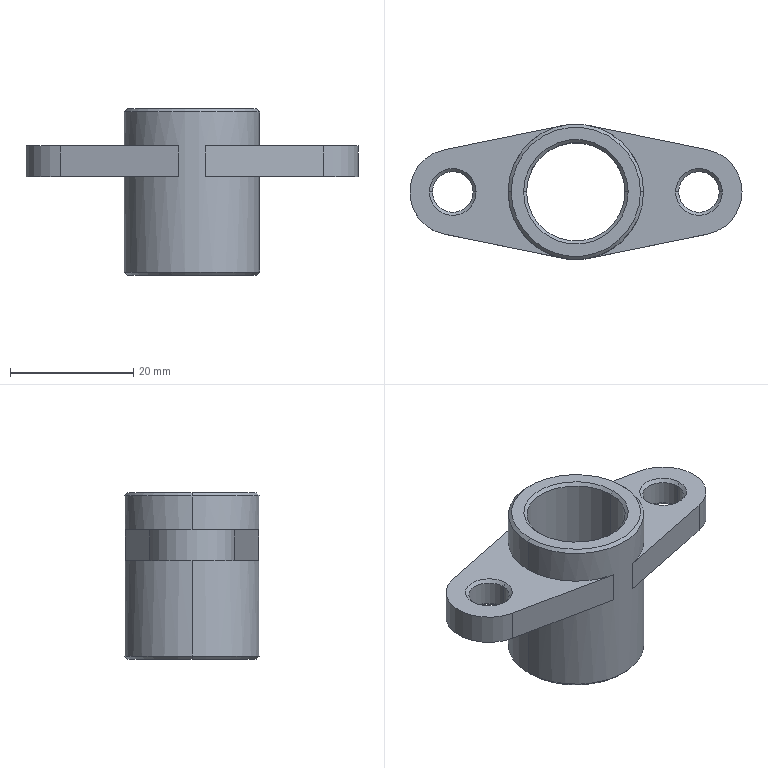Part | SolidWorks | features ICE 3, 3DProfileFeature 1, Chamfer 1, Extrusion 1, HoleWzd 1 | 1 solid | 37 faces | box 54 x 22 x 27 mm | volume 6993 mm3 | cone 16 | cylinder 11 | plane 10 | commonest cylinder face diameters 6.6 x4 14 x3 16 x2 22 x2
STEP:
#1=CARTESIAN_POINT('',(-10.5,0.,0.));
#2=VERTEX_POINT('',#1);
#3=CARTESIAN_POINT('',(10.5,0.,0.));
#4=VERTEX_POINT('',#3);
#5=CARTESIAN_POINT('',(0.,0.,0.));
#6=DIRECTION('',(0.,0.,-1.));
#7=DIRECTION('',(1.,0.,0.));
#8=AXIS2_PLACEMENT_3D('',#5,#6,#7);
#9=CIRCLE('',#8,10.5);
#10=EDGE_CURVE('',#2,#4,#9,.T.);
#11=ORIENTED_EDGE('',*,*,#10,.F.);
#12=CARTESIAN_POINT('',(-11.,0.,0.5));
#13=VERTEX_POINT('',#12);
#14=CARTESIAN_POINT('',(-11.,0.,0.5));
#15=DIRECTION('',(-0.7071,0.,0.7071));
#16=VECTOR('',#15,1000.);
#17=LINE('',#14,#16);
#18=EDGE_CURVE('',#2,#13,#17,.T.);
#19=ORIENTED_EDGE('',*,*,#18,.T.);
#20=CARTESIAN_POINT('',(11.,0.,0.5));
#21=VERTEX_POINT('',#20);
#22=CARTESIAN_POINT('',(0.,0.,0.5));
#23=DIRECTION('',(0.,0.,1.));
#24=DIRECTION('',(1.,0.,0.));
#25=AXIS2_PLACEMENT_3D('',#22,#23,#24);
#26=CIRCLE('',#25,11.);
#27=EDGE_CURVE('',#21,#13,#26,.T.);
#28=ORIENTED_EDGE('',*,*,#27,.F.);
#29=CARTESIAN_POINT('',(11.,0.,0.5));
#30=DIRECTION('',(0.7071,0.,0.7071));
#31=VECTOR('',#30,1000.);
#32=LINE('',#29,#31);
#33=EDGE_CURVE('',#4,#21,#32,.T.);
#34=ORIENTED_EDGE('',*,*,#33,.F.);
#35=EDGE_LOOP('',(#11,#19,#28,#34));
#36=FACE_OUTER_BOUND('',#35,.T.);
#37=CARTESIAN_POINT('',(0.,0.,0.5));
#38=DIRECTION('',(0.,0.,1.));
#39=DIRECTION('',(1.,0.,0.));
#40=AXIS2_PLACEMENT_3D('',#37,#38,#39);
#41=CONICAL_SURFACE('',#40,11.,0.7854);
#42=ADVANCED_FACE('',(#36),#41,.T.);
#43=CARTESIAN_POINT('',(8.,0.,0.5));
#44=VERTEX_POINT('',#43);
#45=CARTESIAN_POINT('',(-8.,0.,0.5));
#46=VERTEX_POINT('',#45);
#47=CARTESIAN_POINT('',(0.,0.,0.5));
#48=DIRECTION('',(0.,0.,-1.));
#49=DIRECTION('',(1.,0.,0.));
#50=AXIS2_PLACEMENT_3D('',#47,#48,#49);
#51=CIRCLE('',#50,8.);
#52=EDGE_CURVE('',#44,#46,#51,.T.);
#53=ORIENTED_EDGE('',*,*,#52,.F.);
#54=CARTESIAN_POINT('',(8.5,0.,0.));
#55=VERTEX_POINT('',#54);
#56=CARTESIAN_POINT('',(8.5,0.,0.));
#57=DIRECTION('',(0.7071,0.,-0.7071));
#58=VECTOR('',#57,1000.);
#59=LINE('',#56,#58);
#60=EDGE_CURVE('',#44,#55,#59,.T.);
#61=ORIENTED_EDGE('',*,*,#60,.T.);
#62=CARTESIAN_POINT('',(-8.5,0.,0.));
#63=VERTEX_POINT('',#62);
#64=CARTESIAN_POINT('',(0.,0.,0.));
#65=DIRECTION('',(0.,0.,1.));
#66=DIRECTION('',(1.,0.,0.));
#67=AXIS2_PLACEMENT_3D('',#64,#65,#66);
#68=CIRCLE('',#67,8.5);
#69=EDGE_CURVE('',#63,#55,#68,.T.);
#70=ORIENTED_EDGE('',*,*,#69,.F.);
#71=CARTESIAN_POINT('',(-8.5,0.,0.));
#72=DIRECTION('',(-0.7071,0.,-0.7071));
#73=VECTOR('',#72,1000.);
#74=LINE('',#71,#73);
#75=EDGE_CURVE('',#46,#63,#74,.T.);
#76=ORIENTED_EDGE('',*,*,#75,.F.);
#77=EDGE_LOOP('',(#53,#61,#70,#76));
#78=FACE_OUTER_BOUND('',#77,.T.);
#79=CARTESIAN_POINT('',(0.,0.,0.));
#80=DIRECTION('',(0.,0.,-1.));
#81=DIRECTION('',(-1.,0.,0.));
#82=AXIS2_PLACEMENT_3D('',#79,#80,#81);
#83=CONICAL_SURFACE('',#82,8.5,0.7854);
#84=ADVANCED_FACE('',(#78),#83,.F.);
#85=CARTESIAN_POINT('',(-16.7,0.,16.5));
#86=VERTEX_POINT('',#85);
#87=CARTESIAN_POINT('',(-23.3,0.,16.5));
#88=VERTEX_POINT('',#87);
#89=CARTESIAN_POINT('',(-20.,0.,16.5));
#90=DIRECTION('',(0.,0.,-1.));
#91=DIRECTION('',(1.,0.,0.));
#92=AXIS2_PLACEMENT_3D('',#89,#90,#91);
#93=CIRCLE('',#92,3.3);
#94=EDGE_CURVE('',#86,#88,#93,.T.);
#95=ORIENTED_EDGE('',*,*,#94,.F.);
#96=CARTESIAN_POINT('',(-16.2,0.,16.));
#97=VERTEX_POINT('',#96);
#98=CARTESIAN_POINT('',(-16.2,0.,16.));
#99=DIRECTION('',(0.7071,0.,-0.7071));
#100=VECTOR('',#99,1000.);
#101=LINE('',#98,#100);
#102=EDGE_CURVE('',#86,#97,#101,.T.);
#103=ORIENTED_EDGE('',*,*,#102,.T.);
#104=CARTESIAN_POINT('',(-23.8,0.,16.));
#105=VERTEX_POINT('',#104);
#106=CARTESIAN_POINT('',(-20.,0.,16.));
#107=DIRECTION('',(0.,0.,1.));
#108=DIRECTION('',(1.,0.,0.));
#109=AXIS2_PLACEMENT_3D('',#106,#107,#108);
#110=CIRCLE('',#109,3.8);
#111=EDGE_CURVE('',#105,#97,#110,.T.);
#112=ORIENTED_EDGE('',*,*,#111,.F.);
#113=CARTESIAN_POINT('',(-23.8,0.,16.));
#114=DIRECTION('',(-0.7071,0.,-0.7071));
#115=VECTOR('',#114,1000.);
#116=LINE('',#113,#115);
#117=EDGE_CURVE('',#88,#105,#116,.T.);
#118=ORIENTED_EDGE('',*,*,#117,.F.);
#119=EDGE_LOOP('',(#95,#103,#112,#118));
#120=FACE_OUTER_BOUND('',#119,.T.);
#121=CARTESIAN_POINT('',(-20.,0.,16.));
#122=DIRECTION('',(0.,0.,-1.));
#123=DIRECTION('',(-1.,0.,0.));
#124=AXIS2_PLACEMENT_3D('',#121,#122,#123);
#125=CONICAL_SURFACE('',#124,3.8,0.7854);
#126=ADVANCED_FACE('',(#120),#125,.F.);
#127=CARTESIAN_POINT('',(-23.3,0.,20.5));
#128=VERTEX_POINT('',#127);
#129=CARTESIAN_POINT('',(-16.7,0.,20.5));
#130=VERTEX_POINT('',#129);
#131=CARTESIAN_POINT('',(-20.,0.,20.5));
#132=DIRECTION('',(0.,0.,1.));
#133=DIRECTION('',(-1.,0.,0.));
#134=AXIS2_PLACEMENT_3D('',#131,#132,#133);
#135=CIRCLE('',#134,3.3);
#136=EDGE_CURVE('',#128,#130,#135,.T.);
#137=ORIENTED_EDGE('',*,*,#136,.F.);
#138=CARTESIAN_POINT('',(-23.8,0.,21.));
#139=VERTEX_POINT('',#138);
#140=CARTESIAN_POINT('',(-23.3,0.,20.5));
#141=DIRECTION('',(-0.7071,0.,0.7071));
#142=VECTOR('',#141,1000.);
#143=LINE('',#140,#142);
#144=EDGE_CURVE('',#128,#139,#143,.T.);
#145=ORIENTED_EDGE('',*,*,#144,.T.);
#146=CARTESIAN_POINT('',(-16.2,0.,21.));
#147=VERTEX_POINT('',#146);
#148=CARTESIAN_POINT('',(-20.,0.,21.));
#149=DIRECTION('',(0.,0.,-1.));
#150=DIRECTION('',(-1.,0.,0.));
#151=AXIS2_PLACEMENT_3D('',#148,#149,#150);
#152=CIRCLE('',#151,3.8);
#153=EDGE_CURVE('',#147,#139,#152,.T.);
#154=ORIENTED_EDGE('',*,*,#153,.F.);
#155=CARTESIAN_POINT('',(-16.7,0.,20.5));
#156=DIRECTION('',(0.7071,0.,0.7071));
#157=VECTOR('',#156,1000.);
#158=LINE('',#155,#157);
#159=EDGE_CURVE('',#130,#147,#158,.T.);
#160=ORIENTED_EDGE('',*,*,#159,.F.);
#161=EDGE_LOOP('',(#137,#145,#154,#160));
#162=FACE_OUTER_BOUND('',#161,.T.);
#163=CARTESIAN_POINT('',(-20.,0.,20.5));
#164=DIRECTION('',(0.,0.,1.));
#165=DIRECTION('',(1.,0.,0.));
#166=AXIS2_PLACEMENT_3D('',#163,#164,#165);
#167=CONICAL_SURFACE('',#166,3.3,0.7854);
#168=ADVANCED_FACE('',(#162),#167,.F.);
#169=CARTESIAN_POINT('',(23.3,0.,16.5));
#170=VERTEX_POINT('',#169);
#171=CARTESIAN_POINT('',(16.7,0.,16.5));
#172=VERTEX_POINT('',#171);
#173=CARTESIAN_POINT('',(20.,0.,16.5));
#174=DIRECTION('',(0.,0.,-1.));
#175=DIRECTION('',(1.,0.,0.));
#176=AXIS2_PLACEMENT_3D('',#173,#174,#175);
#177=CIRCLE('',#176,3.3);
#178=EDGE_CURVE('',#170,#172,#177,.T.);
#179=ORIENTED_EDGE('',*,*,#178,.F.);
#180=CARTESIAN_POINT('',(23.8,0.,16.));
#181=VERTEX_POINT('',#180);
#182=CARTESIAN_POINT('',(23.8,0.,16.));
#183=DIRECTION('',(0.7071,0.,-0.7071));
#184=VECTOR('',#183,1000.);
#185=LINE('',#182,#184);
#186=EDGE_CURVE('',#170,#181,#185,.T.);
#187=ORIENTED_EDGE('',*,*,#186,.T.);
#188=CARTESIAN_POINT('',(16.2,0.,16.));
#189=VERTEX_POINT('',#188);
#190=CARTESIAN_POINT('',(20.,0.,16.));
#191=DIRECTION('',(0.,0.,1.));
#192=DIRECTION('',(1.,0.,0.));
#193=AXIS2_PLACEMENT_3D('',#190,#191,#192);
#194=CIRCLE('',#193,3.8);
#195=EDGE_CURVE('',#189,#181,#194,.T.);
#196=ORIENTED_EDGE('',*,*,#195,.F.);
#197=CARTESIAN_POINT('',(16.2,0.,16.));
#198=DIRECTION('',(-0.7071,0.,-0.7071));
#199=VECTOR('',#198,1000.);
#200=LINE('',#197,#199);
#201=EDGE_CURVE('',#172,#189,#200,.T.);
#202=ORIENTED_EDGE('',*,*,#201,.F.);
#203=EDGE_LOOP('',(#179,#187,#196,#202));
#204=FACE_OUTER_BOUND('',#203,.T.);
#205=CARTESIAN_POINT('',(20.,0.,16.));
#206=DIRECTION('',(0.,0.,-1.));
#207=DIRECTION('',(-1.,0.,0.));
#208=AXIS2_PLACEMENT_3D('',#205,#206,#207);
#209=CONICAL_SURFACE('',#208,3.8,0.7854);
#210=ADVANCED_FACE('',(#204),#209,.F.);
#211=CARTESIAN_POINT('',(16.7,0.,20.5));
#212=VERTEX_POINT('',#211);
#213=CARTESIAN_POINT('',(23.3,0.,20.5));
#214=VERTEX_POINT('',#213);
#215=CARTESIAN_POINT('',(20.,0.,20.5));
#216=DIRECTION('',(0.,0.,1.));
#217=DIRECTION('',(-1.,0.,0.));
#218=AXIS2_PLACEMENT_3D('',#215,#216,#217);
#219=CIRCLE('',#218,3.3);
#220=EDGE_CURVE('',#212,#214,#219,.T.);
#221=ORIENTED_EDGE('',*,*,#220,.F.);
#222=CARTESIAN_POINT('',(16.2,0.,21.));
#223=VERTEX_POINT('',#222);
#224=CARTESIAN_POINT('',(16.7,0.,20.5));
#225=DIRECTION('',(-0.7071,0.,0.7071));
#226=VECTOR('',#225,1000.);
#227=LINE('',#224,#226);
#228=EDGE_CURVE('',#212,#223,#227,.T.);
#229=ORIENTED_EDGE('',*,*,#228,.T.);
#230=CARTESIAN_POINT('',(23.8,0.,21.));
#231=VERTEX_POINT('',#230);
#232=CARTESIAN_POINT('',(20.,0.,21.));
#233=DIRECTION('',(0.,0.,-1.));
#234=DIRECTION('',(-1.,0.,0.));
#235=AXIS2_PLACEMENT_3D('',#232,#233,#234);
#236=CIRCLE('',#235,3.8);
#237=EDGE_CURVE('',#231,#223,#236,.T.);
#238=ORIENTED_EDGE('',*,*,#237,.F.);
#239=CARTESIAN_POINT('',(23.3,0.,20.5));
#240=DIRECTION('',(0.7071,0.,0.7071));
#241=VECTOR('',#240,1000.);
#242=LINE('',#239,#241);
#243=EDGE_CURVE('',#214,#231,#242,.T.);
#244=ORIENTED_EDGE('',*,*,#243,.F.);
#245=EDGE_LOOP('',(#221,#229,#238,#244));
#246=FACE_OUTER_BOUND('',#245,.T.);
#247=CARTESIAN_POINT('',(20.,0.,20.5));
#248=DIRECTION('',(0.,0.,1.));
#249=DIRECTION('',(1.,0.,0.));
#250=AXIS2_PLACEMENT_3D('',#247,#248,#249);
#251=CONICAL_SURFACE('',#250,3.3,0.7854);
#252=ADVANCED_FACE('',(#246),#251,.F.);
#253=CARTESIAN_POINT('',(-8.,0.,26.5));
#254=VERTEX_POINT('',#253);
#255=CARTESIAN_POINT('',(8.,0.,26.5));
#256=VERTEX_POINT('',#255);
#257=CARTESIAN_POINT('',(0.,0.,26.5));
#258=DIRECTION('',(0.,0.,1.));
#259=DIRECTION('',(1.,0.,0.));
#260=AXIS2_PLACEMENT_3D('',#257,#258,#259);
#261=CIRCLE('',#260,8.);
#262=EDGE_CURVE('',#254,#256,#261,.T.);
#263=ORIENTED_EDGE('',*,*,#262,.F.);
#264=CARTESIAN_POINT('',(-8.5,0.,27.));
#265=VERTEX_POINT('',#264);
#266=CARTESIAN_POINT('',(-8.,0.,26.5));
#267=DIRECTION('',(-0.7071,0.,0.7071));
#268=VECTOR('',#267,1000.);
#269=LINE('',#266,#268);
#270=EDGE_CURVE('',#254,#265,#269,.T.);
#271=ORIENTED_EDGE('',*,*,#270,.T.);
#272=CARTESIAN_POINT('',(8.5,0.,27.));
#273=VERTEX_POINT('',#272);
#274=CARTESIAN_POINT('',(0.,0.,27.));
#275=DIRECTION('',(0.,0.,-1.));
#276=DIRECTION('',(1.,0.,0.));
#277=AXIS2_PLACEMENT_3D('',#274,#275,#276);
#278=CIRCLE('',#277,8.5);
#279=EDGE_CURVE('',#273,#265,#278,.T.);
#280=ORIENTED_EDGE('',*,*,#279,.F.);
#281=CARTESIAN_POINT('',(8.,0.,26.5));
#282=DIRECTION('',(0.7071,0.,0.7071));
#283=VECTOR('',#282,1000.);
#284=LINE('',#281,#283);
#285=EDGE_CURVE('',#256,#273,#284,.T.);
#286=ORIENTED_EDGE('',*,*,#285,.F.);
#287=EDGE_LOOP('',(#263,#271,#280,#286));
#288=FACE_OUTER_BOUND('',#287,.T.);
#289=CARTESIAN_POINT('',(0.,0.,26.5));
#290=DIRECTION('',(0.,0.,1.));
#291=DIRECTION('',(1.,0.,0.));
#292=AXIS2_PLACEMENT_3D('',#289,#290,#291);
#293=CONICAL_SURFACE('',#292,8.,0.7854);
#294=ADVANCED_FACE('',(#288),#293,.F.);
#295=CARTESIAN_POINT('',(10.5,0.,27.));
#296=VERTEX_POINT('',#295);
#297=CARTESIAN_POINT('',(-10.5,0.,27.));
#298=VERTEX_POINT('',#297);
#299=CARTESIAN_POINT('',(0.,0.,27.));
#300=DIRECTION('',(0.,0.,1.));
#301=DIRECTION('',(1.,0.,0.));
#302=AXIS2_PLACEMENT_3D('',#299,#300,#301);
#303=CIRCLE('',#302,10.5);
#304=EDGE_CURVE('',#296,#298,#303,.T.);
#305=ORIENTED_EDGE('',*,*,#304,.F.);
#306=CARTESIAN_POINT('',(11.,0.,26.5));
#307=VERTEX_POINT('',#306);
#308=CARTESIAN_POINT('',(10.5,0.,27.));
#309=DIRECTION('',(0.7071,0.,-0.7071));
#310=VECTOR('',#309,1000.);
#311=LINE('',#308,#310);
#312=EDGE_CURVE('',#296,#307,#311,.T.);
#313=ORIENTED_EDGE('',*,*,#312,.T.);
#314=CARTESIAN_POINT('',(-11.,0.,26.5));
#315=VERTEX_POINT('',#314);
#316=CARTESIAN_POINT('',(0.,0.,26.5));
#317=DIRECTION('',(0.,0.,-1.));
#318=DIRECTION('',(1.,0.,0.));
#319=AXIS2_PLACEMENT_3D('',#316,#317,#318);
#320=CIRCLE('',#319,11.);
#321=EDGE_CURVE('',#315,#307,#320,.T.);
#322=ORIENTED_EDGE('',*,*,#321,.F.);
#323=CARTESIAN_POINT('',(-10.5,0.,27.));
#324=DIRECTION('',(-0.7071,0.,-0.7071));
#325=VECTOR('',#324,1000.);
#326=LINE('',#323,#325);
#327=EDGE_CURVE('',#298,#315,#326,.T.);
#328=ORIENTED_EDGE('',*,*,#327,.F.);
#329=EDGE_LOOP('',(#305,#313,#322,#328));
#330=FACE_OUTER_BOUND('',#329,.T.);
#331=CARTESIAN_POINT('',(0.,0.,27.));
#332=DIRECTION('',(0.,0.,-1.));
#333=DIRECTION('',(-1.,0.,0.));
#334=AXIS2_PLACEMENT_3D('',#331,#332,#333);
#335=CONICAL_SURFACE('',#334,10.5,0.7854);
#336=ADVANCED_FACE('',(#330),#335,.T.);
#337=ORIENTED_EDGE('',*,*,#94,.T.);
#338=CARTESIAN_POINT('',(-23.3,0.,30.));
#339=DIRECTION('',(0.,0.,1.));
#340=VECTOR('',#339,1000.);
#341=LINE('',#338,#340);
#342=EDGE_CURVE('',#88,#128,#341,.T.);
#343=ORIENTED_EDGE('',*,*,#342,.T.);
#344=ORIENTED_EDGE('',*,*,#136,.T.);
#345=CARTESIAN_POINT('',(-16.7,0.,30.));
#346=DIRECTION('',(0.,0.,1.));
#347=VECTOR('',#346,1000.);
#348=LINE('',#345,#347);
#349=EDGE_CURVE('',#86,#130,#348,.T.);
#350=ORIENTED_EDGE('',*,*,#349,.F.);
#351=EDGE_LOOP('',(#337,#343,#344,#350));
#352=FACE_OUTER_BOUND('',#351,.T.);
#353=CARTESIAN_POINT('',(-20.,0.,30.));
#354=DIRECTION('',(0.,0.,1.));
#355=DIRECTION('',(1.,0.,0.));
#356=AXIS2_PLACEMENT_3D('',#353,#354,#355);
#357=CYLINDRICAL_SURFACE('',#356,3.3);
#358=ADVANCED_FACE('',(#352),#357,.F.);
#359=ORIENTED_EDGE('',*,*,#178,.T.);
#360=CARTESIAN_POINT('',(16.7,0.,30.));
#361=DIRECTION('',(0.,0.,1.));
#362=VECTOR('',#361,1000.);
#363=LINE('',#360,#362);
#364=EDGE_CURVE('',#172,#212,#363,.T.);
#365=ORIENTED_EDGE('',*,*,#364,.T.);
#366=ORIENTED_EDGE('',*,*,#220,.T.);
#367=CARTESIAN_POINT('',(23.3,0.,30.));
#368=DIRECTION('',(0.,0.,1.));
#369=VECTOR('',#368,1000.);
#370=LINE('',#367,#369);
#371=EDGE_CURVE('',#170,#214,#370,.T.);
#372=ORIENTED_EDGE('',*,*,#371,.F.);
#373=EDGE_LOOP('',(#359,#365,#366,#372));
#374=FACE_OUTER_BOUND('',#373,.T.);
#375=CARTESIAN_POINT('',(20.,0.,30.));
#376=DIRECTION('',(0.,0.,1.));
#377=DIRECTION('',(1.,0.,0.));
#378=AXIS2_PLACEMENT_3D('',#375,#376,#377);
#379=CYLINDRICAL_SURFACE('',#378,3.3);
#380=ADVANCED_FACE('',(#374),#379,.F.);
#381=CARTESIAN_POINT('',(21.4,-6.859,16.));
#382=VERTEX_POINT('',#381);
#383=CARTESIAN_POINT('',(27.,0.,16.));
#384=VERTEX_POINT('',#383);
#385=CARTESIAN_POINT('',(20.,0.,16.));
#386=DIRECTION('',(0.,0.,1.));
#387=DIRECTION('',(1.,0.,0.));
#388=AXIS2_PLACEMENT_3D('',#385,#386,#387);
#389=CIRCLE('',#388,7.);
#390=EDGE_CURVE('',#382,#384,#389,.T.);
#391=ORIENTED_EDGE('',*,*,#390,.T.);
#392=CARTESIAN_POINT('',(27.,0.,21.));
#393=VERTEX_POINT('',#392);
#394=CARTESIAN_POINT('',(27.,0.,16.));
#395=DIRECTION('',(0.,0.,1.));
#396=VECTOR('',#395,1000.);
#397=LINE('',#394,#396);
#398=EDGE_CURVE('',#384,#393,#397,.T.);
#399=ORIENTED_EDGE('',*,*,#398,.T.);
#400=CARTESIAN_POINT('',(21.4,-6.859,21.));
#401=VERTEX_POINT('',#400);
#402=CARTESIAN_POINT('',(20.,0.,21.));
#403=DIRECTION('',(0.,0.,1.));
#404=DIRECTION('',(-1.,0.,0.));
#405=AXIS2_PLACEMENT_3D('',#402,#403,#404);
#406=CIRCLE('',#405,7.);
#407=EDGE_CURVE('',#401,#393,#406,.T.);
#408=ORIENTED_EDGE('',*,*,#407,.F.);
#409=CARTESIAN_POINT('',(21.4,-6.859,16.));
#410=DIRECTION('',(0.,0.,1.));
#411=VECTOR('',#410,1000.);
#412=LINE('',#409,#411);
#413=EDGE_CURVE('',#382,#401,#412,.T.);
#414=ORIENTED_EDGE('',*,*,#413,.F.);
#415=EDGE_LOOP('',(#391,#399,#408,#414));
#416=FACE_OUTER_BOUND('',#415,.T.);
#417=CARTESIAN_POINT('',(20.,0.,16.));
#418=DIRECTION('',(0.,0.,1.));
#419=DIRECTION('',(1.,0.,0.));
#420=AXIS2_PLACEMENT_3D('',#417,#418,#419);
#421=CYLINDRICAL_SURFACE('',#420,7.);
#422=ADVANCED_FACE('',(#416),#421,.T.);
#423=ORIENTED_EDGE('',*,*,#262,.T.);
#424=CARTESIAN_POINT('',(8.,0.,30.));
#425=DIRECTION('',(0.,0.,-1.));
#426=VECTOR('',#425,1000.);
#427=LINE('',#424,#426);
#428=EDGE_CURVE('',#256,#44,#427,.T.);
#429=ORIENTED_EDGE('',*,*,#428,.T.);
#430=ORIENTED_EDGE('',*,*,#52,.T.);
#431=CARTESIAN_POINT('',(-8.,0.,30.));
#432=DIRECTION('',(0.,0.,-1.));
#433=VECTOR('',#432,1000.);
#434=LINE('',#431,#433);
#435=EDGE_CURVE('',#254,#46,#434,.T.);
#436=ORIENTED_EDGE('',*,*,#435,.F.);
#437=EDGE_LOOP('',(#423,#429,#430,#436));
#438=FACE_OUTER_BOUND('',#437,.T.);
#439=CARTESIAN_POINT('',(0.,0.,30.));
#440=DIRECTION('',(0.,0.,-1.));
#441=DIRECTION('',(-1.,0.,0.));
#442=AXIS2_PLACEMENT_3D('',#439,#440,#441);
#443=CYLINDRICAL_SURFACE('',#442,8.);
#444=ADVANCED_FACE('',(#438),#443,.F.);
#445=ORIENTED_EDGE('',*,*,#321,.T.);
#446=CARTESIAN_POINT('',(11.,0.,21.));
#447=VERTEX_POINT('',#446);
#448=CARTESIAN_POINT('',(11.,0.,30.));
#449=DIRECTION('',(0.,0.,-1.));
#450=VECTOR('',#449,1000.);
#451=LINE('',#448,#450);
#452=EDGE_CURVE('',#307,#447,#451,.T.);
#453=ORIENTED_EDGE('',*,*,#452,.T.);
#454=CARTESIAN_POINT('',(2.2,10.778,21.));
#455=VERTEX_POINT('',#454);
#456=CARTESIAN_POINT('',(0.,0.,21.));
#457=DIRECTION('',(0.,0.,1.));
#458=DIRECTION('',(-1.,0.,0.));
#459=AXIS2_PLACEMENT_3D('',#456,#457,#458);
#460=CIRCLE('',#459,11.);
#461=EDGE_CURVE('',#447,#455,#460,.T.);
#462=ORIENTED_EDGE('',*,*,#461,.T.);
#463=CARTESIAN_POINT('',(2.2,10.778,16.));
#464=VERTEX_POINT('',#463);
#465=CARTESIAN_POINT('',(2.2,10.778,16.));
#466=DIRECTION('',(0.,0.,1.));
#467=VECTOR('',#466,1000.);
#468=LINE('',#465,#467);
#469=EDGE_CURVE('',#464,#455,#468,.T.);
#470=ORIENTED_EDGE('',*,*,#469,.F.);
#471=CARTESIAN_POINT('',(11.,0.,16.));
#472=VERTEX_POINT('',#471);
#473=CARTESIAN_POINT('',(0.,0.,16.));
#474=DIRECTION('',(0.,0.,1.));
#475=DIRECTION('',(1.,0.,0.));
#476=AXIS2_PLACEMENT_3D('',#473,#474,#475);
#477=CIRCLE('',#476,11.);
#478=EDGE_CURVE('',#472,#464,#477,.T.);
#479=ORIENTED_EDGE('',*,*,#478,.F.);
#480=CARTESIAN_POINT('',(11.,0.,30.));
#481=DIRECTION('',(0.,0.,-1.));
#482=VECTOR('',#481,1000.);
#483=LINE('',#480,#482);
#484=EDGE_CURVE('',#472,#21,#483,.T.);
#485=ORIENTED_EDGE('',*,*,#484,.T.);
#486=ORIENTED_EDGE('',*,*,#27,.T.);
#487=CARTESIAN_POINT('',(-11.,0.,16.));
#488=VERTEX_POINT('',#487);
#489=CARTESIAN_POINT('',(-11.,0.,30.));
#490=DIRECTION('',(0.,0.,-1.));
#491=VECTOR('',#490,1000.);
#492=LINE('',#489,#491);
#493=EDGE_CURVE('',#488,#13,#492,.T.);
#494=ORIENTED_EDGE('',*,*,#493,.F.);
#495=CARTESIAN_POINT('',(-2.2,10.778,16.));
#496=VERTEX_POINT('',#495);
#497=CARTESIAN_POINT('',(0.,0.,16.));
#498=DIRECTION('',(0.,0.,1.));
#499=DIRECTION('',(1.,0.,0.));
#500=AXIS2_PLACEMENT_3D('',#497,#498,#499);
#501=CIRCLE('',#500,11.);
#502=EDGE_CURVE('',#496,#488,#501,.T.);
#503=ORIENTED_EDGE('',*,*,#502,.F.);
#504=CARTESIAN_POINT('',(-2.2,10.778,21.));
#505=VERTEX_POINT('',#504);
#506=CARTESIAN_POINT('',(-2.2,10.778,16.));
#507=DIRECTION('',(0.,0.,1.));
#508=VECTOR('',#507,1000.);
#509=LINE('',#506,#508);
#510=EDGE_CURVE('',#496,#505,#509,.T.);
#511=ORIENTED_EDGE('',*,*,#510,.T.);
#512=CARTESIAN_POINT('',(-11.,0.,21.));
#513=VERTEX_POINT('',#512);
#514=CARTESIAN_POINT('',(0.,0.,21.));
#515=DIRECTION('',(0.,0.,1.));
#516=DIRECTION('',(-1.,0.,0.));
#517=AXIS2_PLACEMENT_3D('',#514,#515,#516);
#518=CIRCLE('',#517,11.);
#519=EDGE_CURVE('',#505,#513,#518,.T.);
#520=ORIENTED_EDGE('',*,*,#519,.T.);
#521=CARTESIAN_POINT('',(-11.,0.,30.));
#522=DIRECTION('',(0.,0.,-1.));
#523=VECTOR('',#522,1000.);
#524=LINE('',#521,#523);
#525=EDGE_CURVE('',#315,#513,#524,.T.);
#526=ORIENTED_EDGE('',*,*,#525,.F.);
#527=EDGE_LOOP('',(#445,#453,#462,#470,#479,#485,#486,#494,#503,#511,#520,#526));
#528=FACE_OUTER_BOUND('',#527,.T.);
#529=CARTESIAN_POINT('',(0.,0.,30.));
#530=DIRECTION('',(0.,0.,-1.));
#531=DIRECTION('',(-1.,0.,0.));
#532=AXIS2_PLACEMENT_3D('',#529,#530,#531);
#533=CYLINDRICAL_SURFACE('',#532,11.);
#534=ADVANCED_FACE('',(#528),#533,.T.);
#535=ORIENTED_EDGE('',*,*,#452,.F.);
#536=CARTESIAN_POINT('',(0.,0.,26.5));
#537=DIRECTION('',(0.,0.,-1.));
#538=DIRECTION('',(1.,0.,0.));
#539=AXIS2_PLACEMENT_3D('',#536,#537,#538);
#540=CIRCLE('',#539,11.);
#541=EDGE_CURVE('',#307,#315,#540,.T.);
#542=ORIENTED_EDGE('',*,*,#541,.T.);
#543=ORIENTED_EDGE('',*,*,#525,.T.);
#544=CARTESIAN_POINT('',(-2.2,-10.778,21.));
#545=VERTEX_POINT('',#544);
#546=CARTESIAN_POINT('',(0.,0.,21.));
#547=DIRECTION('',(0.,0.,1.));
#548=DIRECTION('',(-1.,0.,0.));
#549=AXIS2_PLACEMENT_3D('',#546,#547,#548);
#550=CIRCLE('',#549,11.);
#551=EDGE_CURVE('',#513,#545,#550,.T.);
#552=ORIENTED_EDGE('',*,*,#551,.T.);
#553=CARTESIAN_POINT('',(-2.2,-10.778,16.));
#554=VERTEX_POINT('',#553);
#555=CARTESIAN_POINT('',(-2.2,-10.778,16.));
#556=DIRECTION('',(0.,0.,1.));
#557=VECTOR('',#556,1000.);
#558=LINE('',#555,#557);
#559=EDGE_CURVE('',#554,#545,#558,.T.);
#560=ORIENTED_EDGE('',*,*,#559,.F.);
#561=CARTESIAN_POINT('',(0.,0.,16.));
#562=DIRECTION('',(0.,0.,1.));
#563=DIRECTION('',(1.,0.,0.));
#564=AXIS2_PLACEMENT_3D('',#561,#562,#563);
#565=CIRCLE('',#564,11.);
#566=EDGE_CURVE('',#488,#554,#565,.T.);
#567=ORIENTED_EDGE('',*,*,#566,.F.);
#568=ORIENTED_EDGE('',*,*,#493,.T.);
#569=CARTESIAN_POINT('',(0.,0.,0.5));
#570=DIRECTION('',(0.,0.,1.));
#571=DIRECTION('',(1.,0.,0.));
#572=AXIS2_PLACEMENT_3D('',#569,#570,#571);
#573=CIRCLE('',#572,11.);
#574=EDGE_CURVE('',#13,#21,#573,.T.);
#575=ORIENTED_EDGE('',*,*,#574,.T.);
#576=ORIENTED_EDGE('',*,*,#484,.F.);
#577=CARTESIAN_POINT('',(2.2,-10.778,16.));
#578=VERTEX_POINT('',#577);
#579=CARTESIAN_POINT('',(0.,0.,16.));
#580=DIRECTION('',(0.,0.,1.));
#581=DIRECTION('',(1.,0.,0.));
#582=AXIS2_PLACEMENT_3D('',#579,#580,#581);
#583=CIRCLE('',#582,11.);
#584=EDGE_CURVE('',#578,#472,#583,.T.);
#585=ORIENTED_EDGE('',*,*,#584,.F.);
#586=CARTESIAN_POINT('',(2.2,-10.778,21.));
#587=VERTEX_POINT('',#586);
#588=CARTESIAN_POINT('',(2.2,-10.778,16.));
#589=DIRECTION('',(0.,0.,1.));
#590=VECTOR('',#589,1000.);
#591=LINE('',#588,#590);
#592=EDGE_CURVE('',#578,#587,#591,.T.);
#593=ORIENTED_EDGE('',*,*,#592,.T.);
#594=CARTESIAN_POINT('',(0.,0.,21.));
#595=DIRECTION('',(0.,0.,1.));
#596=DIRECTION('',(-1.,0.,0.));
#597=AXIS2_PLACEMENT_3D('',#594,#595,#596);
#598=CIRCLE('',#597,11.);
#599=EDGE_CURVE('',#587,#447,#598,.T.);
#600=ORIENTED_EDGE('',*,*,#599,.T.);
#601=EDGE_LOOP('',(#535,#542,#543,#552,#560,#567,#568,#575,#576,#585,#593,#600));
#602=FACE_OUTER_BOUND('',#601,.T.);
#603=CARTESIAN_POINT('',(0.,0.,30.));
#604=DIRECTION('',(0.,0.,-1.));
#605=DIRECTION('',(-1.,0.,0.));
#606=AXIS2_PLACEMENT_3D('',#603,#604,#605);
#607=CYLINDRICAL_SURFACE('',#606,11.);
#608=ADVANCED_FACE('',(#602),#607,.T.);
#609=ORIENTED_EDGE('',*,*,#428,.F.);
#610=CARTESIAN_POINT('',(0.,0.,26.5));
#611=DIRECTION('',(0.,0.,1.));
#612=DIRECTION('',(1.,0.,0.));
#613=AXIS2_PLACEMENT_3D('',#610,#611,#612);
#614=CIRCLE('',#613,8.);
#615=EDGE_CURVE('',#256,#254,#614,.T.);
#616=ORIENTED_EDGE('',*,*,#615,.T.);
#617=ORIENTED_EDGE('',*,*,#435,.T.);
#618=CARTESIAN_POINT('',(0.,0.,0.5));
#619=DIRECTION('',(0.,0.,-1.));
#620=DIRECTION('',(1.,0.,0.));
#621=AXIS2_PLACEMENT_3D('',#618,#619,#620);
#622=CIRCLE('',#621,8.);
#623=EDGE_CURVE('',#46,#44,#622,.T.);
#624=ORIENTED_EDGE('',*,*,#623,.T.);
#625=EDGE_LOOP('',(#609,#616,#617,#624));
#626=FACE_OUTER_BOUND('',#625,.T.);
#627=CARTESIAN_POINT('',(0.,0.,30.));
#628=DIRECTION('',(0.,0.,-1.));
#629=DIRECTION('',(-1.,0.,0.));
#630=AXIS2_PLACEMENT_3D('',#627,#628,#629);
#631=CYLINDRICAL_SURFACE('',#630,8.);
#632=ADVANCED_FACE('',(#626),#631,.F.);
#633=ORIENTED_EDGE('',*,*,#69,.T.);
#634=CARTESIAN_POINT('',(0.,0.,0.));
#635=DIRECTION('',(0.,0.,1.));
#636=DIRECTION('',(1.,0.,0.));
#637=AXIS2_PLACEMENT_3D('',#634,#635,#636);
#638=CIRCLE('',#637,8.5);
#639=EDGE_CURVE('',#55,#63,#638,.T.);
#640=ORIENTED_EDGE('',*,*,#639,.T.);
#641=EDGE_LOOP('',(#633,#640));
#642=FACE_BOUND('',#641,.T.);
#643=CARTESIAN_POINT('',(0.,0.,0.));
#644=DIRECTION('',(0.,0.,-1.));
#645=DIRECTION('',(1.,0.,0.));
#646=AXIS2_PLACEMENT_3D('',#643,#644,#645);
#647=CIRCLE('',#646,10.5);
#648=EDGE_CURVE('',#4,#2,#647,.T.);
#649=ORIENTED_EDGE('',*,*,#648,.T.);
#650=ORIENTED_EDGE('',*,*,#10,.T.);
#651=EDGE_LOOP('',(#649,#650));
#652=FACE_OUTER_BOUND('',#651,.T.);
#653=CARTESIAN_POINT('',(0.,0.,0.));
#654=DIRECTION('',(0.,0.,1.));
#655=DIRECTION('',(1.,0.,0.));
#656=AXIS2_PLACEMENT_3D('',#653,#654,#655);
#657=PLANE('',#656);
#658=ADVANCED_FACE('',(#642,#652),#657,.F.);
#659=ORIENTED_EDGE('',*,*,#398,.F.);
#660=CARTESIAN_POINT('',(21.4,6.859,16.));
#661=VERTEX_POINT('',#660);
#662=CARTESIAN_POINT('',(20.,0.,16.));
#663=DIRECTION('',(0.,0.,1.));
#664=DIRECTION('',(1.,0.,0.));
#665=AXIS2_PLACEMENT_3D('',#662,#663,#664);
#666=CIRCLE('',#665,7.);
#667=EDGE_CURVE('',#384,#661,#666,.T.);
#668=ORIENTED_EDGE('',*,*,#667,.T.);
#669=CARTESIAN_POINT('',(21.4,6.859,21.));
#670=VERTEX_POINT('',#669);
#671=CARTESIAN_POINT('',(21.4,6.859,16.));
#672=DIRECTION('',(0.,0.,1.));
#673=VECTOR('',#672,1000.);
#674=LINE('',#671,#673);
#675=EDGE_CURVE('',#661,#670,#674,.T.);
#676=ORIENTED_EDGE('',*,*,#675,.T.);
#677=CARTESIAN_POINT('',(20.,0.,21.));
#678=DIRECTION('',(0.,0.,1.));
#679=DIRECTION('',(-1.,0.,0.));
#680=AXIS2_PLACEMENT_3D('',#677,#678,#679);
#681=CIRCLE('',#680,7.);
#682=EDGE_CURVE('',#393,#670,#681,.T.);
#683=ORIENTED_EDGE('',*,*,#682,.F.);
#684=EDGE_LOOP('',(#659,#668,#676,#683));
#685=FACE_OUTER_BOUND('',#684,.T.);
#686=CARTESIAN_POINT('',(20.,0.,16.));
#687=DIRECTION('',(0.,0.,1.));
#688=DIRECTION('',(1.,0.,0.));
#689=AXIS2_PLACEMENT_3D('',#686,#687,#688);
#690=CYLINDRICAL_SURFACE('',#689,7.);
#691=ADVANCED_FACE('',(#685),#690,.T.);
#692=ORIENTED_EDGE('',*,*,#195,.T.);
#693=CARTESIAN_POINT('',(20.,0.,16.));
#694=DIRECTION('',(0.,0.,1.));
#695=DIRECTION('',(1.,0.,0.));
#696=AXIS2_PLACEMENT_3D('',#693,#694,#695);
#697=CIRCLE('',#696,3.8);
#698=EDGE_CURVE('',#181,#189,#697,.T.);
#699=ORIENTED_EDGE('',*,*,#698,.T.);
#700=EDGE_LOOP('',(#692,#699));
#701=FACE_BOUND('',#700,.T.);
#702=CARTESIAN_POINT('',(2.2,-10.778,16.));
#703=DIRECTION('',(0.9798,0.2,0.));
#704=VECTOR('',#703,1000.);
#705=LINE('',#702,#704);
#706=EDGE_CURVE('',#578,#382,#705,.T.);
#707=ORIENTED_EDGE('',*,*,#706,.F.);
#708=ORIENTED_EDGE('',*,*,#584,.T.);
#709=ORIENTED_EDGE('',*,*,#478,.T.);
#710=CARTESIAN_POINT('',(2.2,10.778,16.));
#711=DIRECTION('',(-0.9798,0.2,0.));
#712=VECTOR('',#711,1000.);
#713=LINE('',#710,#712);
#714=EDGE_CURVE('',#661,#464,#713,.T.);
#715=ORIENTED_EDGE('',*,*,#714,.F.);
#716=ORIENTED_EDGE('',*,*,#667,.F.);
#717=ORIENTED_EDGE('',*,*,#390,.F.);
#718=EDGE_LOOP('',(#707,#708,#709,#715,#716,#717));
#719=FACE_OUTER_BOUND('',#718,.T.);
#720=CARTESIAN_POINT('',(0.,0.,16.));
#721=DIRECTION('',(0.,0.,1.));
#722=DIRECTION('',(1.,0.,0.));
#723=AXIS2_PLACEMENT_3D('',#720,#721,#722);
#724=PLANE('',#723);
#725=ADVANCED_FACE('',(#701,#719),#724,.F.);
#726=CARTESIAN_POINT('',(2.2,-10.778,21.));
#727=DIRECTION('',(0.9798,0.2,0.));
#728=VECTOR('',#727,1000.);
#729=LINE('',#726,#728);
#730=EDGE_CURVE('',#587,#401,#729,.T.);
#731=ORIENTED_EDGE('',*,*,#730,.F.);
#732=ORIENTED_EDGE('',*,*,#592,.F.);
#733=ORIENTED_EDGE('',*,*,#706,.T.);
#734=ORIENTED_EDGE('',*,*,#413,.T.);
#735=EDGE_LOOP('',(#731,#732,#733,#734));
#736=FACE_OUTER_BOUND('',#735,.T.);
#737=CARTESIAN_POINT('',(2.2,-10.778,16.));
#738=DIRECTION('',(0.2,-0.9798,0.));
#739=DIRECTION('',(0.9798,0.2,0.));
#740=AXIS2_PLACEMENT_3D('',#737,#738,#739);
#741=PLANE('',#740);
#742=ADVANCED_FACE('',(#736),#741,.T.);
#743=ORIENTED_EDGE('',*,*,#469,.T.);
#744=CARTESIAN_POINT('',(2.2,10.778,21.));
#745=DIRECTION('',(-0.9798,0.2,0.));
#746=VECTOR('',#745,1000.);
#747=LINE('',#744,#746);
#748=EDGE_CURVE('',#670,#455,#747,.T.);
#749=ORIENTED_EDGE('',*,*,#748,.F.);
#750=ORIENTED_EDGE('',*,*,#675,.F.);
#751=ORIENTED_EDGE('',*,*,#714,.T.);
#752=EDGE_LOOP('',(#743,#749,#750,#751));
#753=FACE_OUTER_BOUND('',#752,.T.);
#754=CARTESIAN_POINT('',(2.2,10.778,16.));
#755=DIRECTION('',(0.2,0.9798,0.));
#756=DIRECTION('',(-0.9798,0.2,0.));
#757=AXIS2_PLACEMENT_3D('',#754,#755,#756);
#758=PLANE('',#757);
#759=ADVANCED_FACE('',(#753),#758,.T.);
#760=ORIENTED_EDGE('',*,*,#111,.T.);
#761=CARTESIAN_POINT('',(-20.,0.,16.));
#762=DIRECTION('',(0.,0.,1.));
#763=DIRECTION('',(1.,0.,0.));
#764=AXIS2_PLACEMENT_3D('',#761,#762,#763);
#765=CIRCLE('',#764,3.8);
#766=EDGE_CURVE('',#97,#105,#765,.T.);
#767=ORIENTED_EDGE('',*,*,#766,.T.);
#768=EDGE_LOOP('',(#760,#767));
#769=FACE_BOUND('',#768,.T.);
#770=CARTESIAN_POINT('',(-21.4,6.859,16.));
#771=VERTEX_POINT('',#770);
#772=CARTESIAN_POINT('',(-21.4,6.859,16.));
#773=DIRECTION('',(-0.9798,-0.2,0.));
#774=VECTOR('',#773,1000.);
#775=LINE('',#772,#774);
#776=EDGE_CURVE('',#496,#771,#775,.T.);
#777=ORIENTED_EDGE('',*,*,#776,.F.);
#778=ORIENTED_EDGE('',*,*,#502,.T.);
#779=ORIENTED_EDGE('',*,*,#566,.T.);
#780=CARTESIAN_POINT('',(-21.4,-6.859,16.));
#781=VERTEX_POINT('',#780);
#782=CARTESIAN_POINT('',(-21.4,-6.859,16.));
#783=DIRECTION('',(0.9798,-0.2,0.));
#784=VECTOR('',#783,1000.);
#785=LINE('',#782,#784);
#786=EDGE_CURVE('',#781,#554,#785,.T.);
#787=ORIENTED_EDGE('',*,*,#786,.F.);
#788=CARTESIAN_POINT('',(-20.,0.,16.));
#789=DIRECTION('',(0.,0.,1.));
#790=DIRECTION('',(1.,0.,0.));
#791=AXIS2_PLACEMENT_3D('',#788,#789,#790);
#792=CIRCLE('',#791,7.);
#793=EDGE_CURVE('',#771,#781,#792,.T.);
#794=ORIENTED_EDGE('',*,*,#793,.F.);
#795=EDGE_LOOP('',(#777,#778,#779,#787,#794));
#796=FACE_OUTER_BOUND('',#795,.T.);
#797=CARTESIAN_POINT('',(0.,0.,16.));
#798=DIRECTION('',(0.,0.,1.));
#799=DIRECTION('',(1.,0.,0.));
#800=AXIS2_PLACEMENT_3D('',#797,#798,#799);
#801=PLANE('',#800);
#802=ADVANCED_FACE('',(#769,#796),#801,.F.);
#803=ORIENTED_EDGE('',*,*,#559,.T.);
#804=CARTESIAN_POINT('',(-21.4,-6.859,21.));
#805=VERTEX_POINT('',#804);
#806=CARTESIAN_POINT('',(-21.4,-6.859,21.));
#807=DIRECTION('',(0.9798,-0.2,0.));
#808=VECTOR('',#807,1000.);
#809=LINE('',#806,#808);
#810=EDGE_CURVE('',#805,#545,#809,.T.);
#811=ORIENTED_EDGE('',*,*,#810,.F.);
#812=CARTESIAN_POINT('',(-21.4,-6.859,16.));
#813=DIRECTION('',(0.,0.,1.));
#814=VECTOR('',#813,1000.);
#815=LINE('',#812,#814);
#816=EDGE_CURVE('',#781,#805,#815,.T.);
#817=ORIENTED_EDGE('',*,*,#816,.F.);
#818=ORIENTED_EDGE('',*,*,#786,.T.);
#819=EDGE_LOOP('',(#803,#811,#817,#818));
#820=FACE_OUTER_BOUND('',#819,.T.);
#821=CARTESIAN_POINT('',(-21.4,-6.859,16.));
#822=DIRECTION('',(-0.2,-0.9798,0.));
#823=DIRECTION('',(0.9798,-0.2,0.));
#824=AXIS2_PLACEMENT_3D('',#821,#822,#823);
#825=PLANE('',#824);
#826=ADVANCED_FACE('',(#820),#825,.T.);
#827=CARTESIAN_POINT('',(-21.4,6.859,21.));
#828=VERTEX_POINT('',#827);
#829=CARTESIAN_POINT('',(-20.,0.,21.));
#830=DIRECTION('',(0.,0.,1.));
#831=DIRECTION('',(-1.,0.,0.));
#832=AXIS2_PLACEMENT_3D('',#829,#830,#831);
#833=CIRCLE('',#832,7.);
#834=EDGE_CURVE('',#828,#805,#833,.T.);
#835=ORIENTED_EDGE('',*,*,#834,.F.);
#836=CARTESIAN_POINT('',(-21.4,6.859,16.));
#837=DIRECTION('',(0.,0.,1.));
#838=VECTOR('',#837,1000.);
#839=LINE('',#836,#838);
#840=EDGE_CURVE('',#771,#828,#839,.T.);
#841=ORIENTED_EDGE('',*,*,#840,.F.);
#842=ORIENTED_EDGE('',*,*,#793,.T.);
#843=ORIENTED_EDGE('',*,*,#816,.T.);
#844=EDGE_LOOP('',(#835,#841,#842,#843));
#845=FACE_OUTER_BOUND('',#844,.T.);
#846=CARTESIAN_POINT('',(-20.,0.,16.));
#847=DIRECTION('',(0.,0.,1.));
#848=DIRECTION('',(1.,0.,0.));
#849=AXIS2_PLACEMENT_3D('',#846,#847,#848);
#850=CYLINDRICAL_SURFACE('',#849,7.);
#851=ADVANCED_FACE('',(#845),#850,.T.);
#852=CARTESIAN_POINT('',(-21.4,6.859,21.));
#853=DIRECTION('',(-0.9798,-0.2,0.));
#854=VECTOR('',#853,1000.);
#855=LINE('',#852,#854);
#856=EDGE_CURVE('',#505,#828,#855,.T.);
#857=ORIENTED_EDGE('',*,*,#856,.F.);
#858=ORIENTED_EDGE('',*,*,#510,.F.);
#859=ORIENTED_EDGE('',*,*,#776,.T.);
#860=ORIENTED_EDGE('',*,*,#840,.T.);
#861=EDGE_LOOP('',(#857,#858,#859,#860));
#862=FACE_OUTER_BOUND('',#861,.T.);
#863=CARTESIAN_POINT('',(-21.4,6.859,16.));
#864=DIRECTION('',(-0.2,0.9798,0.));
#865=DIRECTION('',(-0.9798,-0.2,0.));
#866=AXIS2_PLACEMENT_3D('',#863,#864,#865);
#867=PLANE('',#866);
#868=ADVANCED_FACE('',(#862),#867,.T.);
#869=ORIENTED_EDGE('',*,*,#364,.F.);
#870=CARTESIAN_POINT('',(20.,0.,16.5));
#871=DIRECTION('',(0.,0.,-1.));
#872=DIRECTION('',(1.,0.,0.));
#873=AXIS2_PLACEMENT_3D('',#870,#871,#872);
#874=CIRCLE('',#873,3.3);
#875=EDGE_CURVE('',#172,#170,#874,.T.);
#876=ORIENTED_EDGE('',*,*,#875,.T.);
#877=ORIENTED_EDGE('',*,*,#371,.T.);
#878=CARTESIAN_POINT('',(20.,0.,20.5));
#879=DIRECTION('',(0.,0.,1.));
#880=DIRECTION('',(-1.,0.,0.));
#881=AXIS2_PLACEMENT_3D('',#878,#879,#880);
#882=CIRCLE('',#881,3.3);
#883=EDGE_CURVE('',#214,#212,#882,.T.);
#884=ORIENTED_EDGE('',*,*,#883,.T.);
#885=EDGE_LOOP('',(#869,#876,#877,#884));
#886=FACE_OUTER_BOUND('',#885,.T.);
#887=CARTESIAN_POINT('',(20.,0.,30.));
#888=DIRECTION('',(0.,0.,1.));
#889=DIRECTION('',(1.,0.,0.));
#890=AXIS2_PLACEMENT_3D('',#887,#888,#889);
#891=CYLINDRICAL_SURFACE('',#890,3.3);
#892=ADVANCED_FACE('',(#886),#891,.F.);
#893=ORIENTED_EDGE('',*,*,#237,.T.);
#894=CARTESIAN_POINT('',(20.,0.,21.));
#895=DIRECTION('',(0.,0.,-1.));
#896=DIRECTION('',(-1.,0.,0.));
#897=AXIS2_PLACEMENT_3D('',#894,#895,#896);
#898=CIRCLE('',#897,3.8);
#899=EDGE_CURVE('',#223,#231,#898,.T.);
#900=ORIENTED_EDGE('',*,*,#899,.T.);
#901=EDGE_LOOP('',(#893,#900));
#902=FACE_BOUND('',#901,.T.);
#903=ORIENTED_EDGE('',*,*,#748,.T.);
#904=ORIENTED_EDGE('',*,*,#461,.F.);
#905=ORIENTED_EDGE('',*,*,#599,.F.);
#906=ORIENTED_EDGE('',*,*,#730,.T.);
#907=ORIENTED_EDGE('',*,*,#407,.T.);
#908=ORIENTED_EDGE('',*,*,#682,.T.);
#909=EDGE_LOOP('',(#903,#904,#905,#906,#907,#908));
#910=FACE_OUTER_BOUND('',#909,.T.);
#911=CARTESIAN_POINT('',(23.3,0.,21.));
#912=DIRECTION('',(0.,0.,-1.));
#913=DIRECTION('',(-1.,0.,0.));
#914=AXIS2_PLACEMENT_3D('',#911,#912,#913);
#915=PLANE('',#914);
#916=ADVANCED_FACE('',(#902,#910),#915,.F.);
#917=ORIENTED_EDGE('',*,*,#342,.F.);
#918=CARTESIAN_POINT('',(-20.,0.,16.5));
#919=DIRECTION('',(0.,0.,-1.));
#920=DIRECTION('',(1.,0.,0.));
#921=AXIS2_PLACEMENT_3D('',#918,#919,#920);
#922=CIRCLE('',#921,3.3);
#923=EDGE_CURVE('',#88,#86,#922,.T.);
#924=ORIENTED_EDGE('',*,*,#923,.T.);
#925=ORIENTED_EDGE('',*,*,#349,.T.);
#926=CARTESIAN_POINT('',(-20.,0.,20.5));
#927=DIRECTION('',(0.,0.,1.));
#928=DIRECTION('',(-1.,0.,0.));
#929=AXIS2_PLACEMENT_3D('',#926,#927,#928);
#930=CIRCLE('',#929,3.3);
#931=EDGE_CURVE('',#130,#128,#930,.T.);
#932=ORIENTED_EDGE('',*,*,#931,.T.);
#933=EDGE_LOOP('',(#917,#924,#925,#932));
#934=FACE_OUTER_BOUND('',#933,.T.);
#935=CARTESIAN_POINT('',(-20.,0.,30.));
#936=DIRECTION('',(0.,0.,1.));
#937=DIRECTION('',(1.,0.,0.));
#938=AXIS2_PLACEMENT_3D('',#935,#936,#937);
#939=CYLINDRICAL_SURFACE('',#938,3.3);
#940=ADVANCED_FACE('',(#934),#939,.F.);
#941=ORIENTED_EDGE('',*,*,#153,.T.);
#942=CARTESIAN_POINT('',(-20.,0.,21.));
#943=DIRECTION('',(0.,0.,-1.));
#944=DIRECTION('',(-1.,0.,0.));
#945=AXIS2_PLACEMENT_3D('',#942,#943,#944);
#946=CIRCLE('',#945,3.8);
#947=EDGE_CURVE('',#139,#147,#946,.T.);
#948=ORIENTED_EDGE('',*,*,#947,.T.);
#949=EDGE_LOOP('',(#941,#948));
#950=FACE_BOUND('',#949,.T.);
#951=ORIENTED_EDGE('',*,*,#810,.T.);
#952=ORIENTED_EDGE('',*,*,#551,.F.);
#953=ORIENTED_EDGE('',*,*,#519,.F.);
#954=ORIENTED_EDGE('',*,*,#856,.T.);
#955=ORIENTED_EDGE('',*,*,#834,.T.);
#956=EDGE_LOOP('',(#951,#952,#953,#954,#955));
#957=FACE_OUTER_BOUND('',#956,.T.);
#958=CARTESIAN_POINT('',(-16.7,0.,21.));
#959=DIRECTION('',(0.,0.,-1.));
#960=DIRECTION('',(-1.,0.,0.));
#961=AXIS2_PLACEMENT_3D('',#958,#959,#960);
#962=PLANE('',#961);
#963=ADVANCED_FACE('',(#950,#957),#962,.F.);
#964=CARTESIAN_POINT('',(0.,0.,27.));
#965=DIRECTION('',(0.,0.,1.));
#966=DIRECTION('',(1.,0.,0.));
#967=AXIS2_PLACEMENT_3D('',#964,#965,#966);
#968=CIRCLE('',#967,10.5);
#969=EDGE_CURVE('',#298,#296,#968,.T.);
#970=ORIENTED_EDGE('',*,*,#969,.T.);
#971=ORIENTED_EDGE('',*,*,#304,.T.);
#972=EDGE_LOOP('',(#970,#971));
#973=FACE_OUTER_BOUND('',#972,.T.);
#974=ORIENTED_EDGE('',*,*,#279,.T.);
#975=CARTESIAN_POINT('',(0.,0.,27.));
#976=DIRECTION('',(0.,0.,-1.));
#977=DIRECTION('',(1.,0.,0.));
#978=AXIS2_PLACEMENT_3D('',#975,#976,#977);
#979=CIRCLE('',#978,8.5);
#980=EDGE_CURVE('',#265,#273,#979,.T.);
#981=ORIENTED_EDGE('',*,*,#980,.T.);
#982=EDGE_LOOP('',(#974,#981));
#983=FACE_BOUND('',#982,.T.);
#984=CARTESIAN_POINT('',(0.,0.,27.));
#985=DIRECTION('',(0.,0.,1.));
#986=DIRECTION('',(1.,0.,0.));
#987=AXIS2_PLACEMENT_3D('',#984,#985,#986);
#988=PLANE('',#987);
#989=ADVANCED_FACE('',(#973,#983),#988,.T.);
#990=ORIENTED_EDGE('',*,*,#312,.F.);
#991=ORIENTED_EDGE('',*,*,#969,.F.);
#992=ORIENTED_EDGE('',*,*,#327,.T.);
#993=ORIENTED_EDGE('',*,*,#541,.F.);
#994=EDGE_LOOP('',(#990,#991,#992,#993));
#995=FACE_OUTER_BOUND('',#994,.T.);
#996=CARTESIAN_POINT('',(0.,0.,27.));
#997=DIRECTION('',(0.,0.,-1.));
#998=DIRECTION('',(-1.,0.,0.));
#999=AXIS2_PLACEMENT_3D('',#996,#997,#998);
#1000=CONICAL_SURFACE('',#999,10.5,0.7854);
#1001=ADVANCED_FACE('',(#995),#1000,.T.);
#1002=ORIENTED_EDGE('',*,*,#270,.F.);
#1003=ORIENTED_EDGE('',*,*,#615,.F.);
#1004=ORIENTED_EDGE('',*,*,#285,.T.);
#1005=ORIENTED_EDGE('',*,*,#980,.F.);
#1006=EDGE_LOOP('',(#1002,#1003,#1004,#1005));
#1007=FACE_OUTER_BOUND('',#1006,.T.);
#1008=CARTESIAN_POINT('',(0.,0.,26.5));
#1009=DIRECTION('',(0.,0.,1.));
#1010=DIRECTION('',(1.,0.,0.));
#1011=AXIS2_PLACEMENT_3D('',#1008,#1009,#1010);
#1012=CONICAL_SURFACE('',#1011,8.,0.7854);
#1013=ADVANCED_FACE('',(#1007),#1012,.F.);
#1014=ORIENTED_EDGE('',*,*,#228,.F.);
#1015=ORIENTED_EDGE('',*,*,#883,.F.);
#1016=ORIENTED_EDGE('',*,*,#243,.T.);
#1017=ORIENTED_EDGE('',*,*,#899,.F.);
#1018=EDGE_LOOP('',(#1014,#1015,#1016,#1017));
#1019=FACE_OUTER_BOUND('',#1018,.T.);
#1020=CARTESIAN_POINT('',(20.,0.,20.5));
#1021=DIRECTION('',(0.,0.,1.));
#1022=DIRECTION('',(1.,0.,0.));
#1023=AXIS2_PLACEMENT_3D('',#1020,#1021,#1022);
#1024=CONICAL_SURFACE('',#1023,3.3,0.7854);
#1025=ADVANCED_FACE('',(#1019),#1024,.F.);
#1026=ORIENTED_EDGE('',*,*,#186,.F.);
#1027=ORIENTED_EDGE('',*,*,#875,.F.);
#1028=ORIENTED_EDGE('',*,*,#201,.T.);
#1029=ORIENTED_EDGE('',*,*,#698,.F.);
#1030=EDGE_LOOP('',(#1026,#1027,#1028,#1029));
#1031=FACE_OUTER_BOUND('',#1030,.T.);
#1032=CARTESIAN_POINT('',(20.,0.,16.));
#1033=DIRECTION('',(0.,0.,-1.));
#1034=DIRECTION('',(-1.,0.,0.));
#1035=AXIS2_PLACEMENT_3D('',#1032,#1033,#1034);
#1036=CONICAL_SURFACE('',#1035,3.8,0.7854);
#1037=ADVANCED_FACE('',(#1031),#1036,.F.);
#1038=ORIENTED_EDGE('',*,*,#144,.F.);
#1039=ORIENTED_EDGE('',*,*,#931,.F.);
#1040=ORIENTED_EDGE('',*,*,#159,.T.);
#1041=ORIENTED_EDGE('',*,*,#947,.F.);
#1042=EDGE_LOOP('',(#1038,#1039,#1040,#1041));
#1043=FACE_OUTER_BOUND('',#1042,.T.);
#1044=CARTESIAN_POINT('',(-20.,0.,20.5));
#1045=DIRECTION('',(0.,0.,1.));
#1046=DIRECTION('',(1.,0.,0.));
#1047=AXIS2_PLACEMENT_3D('',#1044,#1045,#1046);
#1048=CONICAL_SURFACE('',#1047,3.3,0.7854);
#1049=ADVANCED_FACE('',(#1043),#1048,.F.);
#1050=ORIENTED_EDGE('',*,*,#102,.F.);
#1051=ORIENTED_EDGE('',*,*,#923,.F.);
#1052=ORIENTED_EDGE('',*,*,#117,.T.);
#1053=ORIENTED_EDGE('',*,*,#766,.F.);
#1054=EDGE_LOOP('',(#1050,#1051,#1052,#1053));
#1055=FACE_OUTER_BOUND('',#1054,.T.);
#1056=CARTESIAN_POINT('',(-20.,0.,16.));
#1057=DIRECTION('',(0.,0.,-1.));
#1058=DIRECTION('',(-1.,0.,0.));
#1059=AXIS2_PLACEMENT_3D('',#1056,#1057,#1058);
#1060=CONICAL_SURFACE('',#1059,3.8,0.7854);
#1061=ADVANCED_FACE('',(#1055),#1060,.F.);
#1062=ORIENTED_EDGE('',*,*,#60,.F.);
#1063=ORIENTED_EDGE('',*,*,#623,.F.);
#1064=ORIENTED_EDGE('',*,*,#75,.T.);
#1065=ORIENTED_EDGE('',*,*,#639,.F.);
#1066=EDGE_LOOP('',(#1062,#1063,#1064,#1065));
#1067=FACE_OUTER_BOUND('',#1066,.T.);
#1068=CARTESIAN_POINT('',(0.,0.,0.));
#1069=DIRECTION('',(0.,0.,-1.));
#1070=DIRECTION('',(-1.,0.,0.));
#1071=AXIS2_PLACEMENT_3D('',#1068,#1069,#1070);
#1072=CONICAL_SURFACE('',#1071,8.5,0.7854);
#1073=ADVANCED_FACE('',(#1067),#1072,.F.);
#1074=ORIENTED_EDGE('',*,*,#18,.F.);
#1075=ORIENTED_EDGE('',*,*,#648,.F.);
#1076=ORIENTED_EDGE('',*,*,#33,.T.);
#1077=ORIENTED_EDGE('',*,*,#574,.F.);
#1078=EDGE_LOOP('',(#1074,#1075,#1076,#1077));
#1079=FACE_OUTER_BOUND('',#1078,.T.);
#1080=CARTESIAN_POINT('',(0.,0.,0.5));
#1081=DIRECTION('',(0.,0.,1.));
#1082=DIRECTION('',(1.,0.,0.));
#1083=AXIS2_PLACEMENT_3D('',#1080,#1081,#1082);
#1084=CONICAL_SURFACE('',#1083,11.,0.7854);
#1085=ADVANCED_FACE('',(#1079),#1084,.T.);
#1086=CLOSED_SHELL('',(#42,#84,#126,#168,#210,#252,#294,#336,#358,#380,#422,#444,#534,#608,#632,#658,#691,#725,#742,#759,#802,#826,#851,#868,#892,#916,#940,#963,#989,#1001,#1013,#1025,#1037,#1049,#1061,#1073,#1085));
#1087=MANIFOLD_SOLID_BREP('',#1086);
#1088=CARTESIAN_POINT('',(0.,0.,0.));
#1089=DIRECTION('',(0.,0.,1.));
#1090=DIRECTION('',(1.,0.,0.));
#1091=AXIS2_PLACEMENT_3D('',#1088,#1089,#1090);
#1092=(LENGTH_UNIT()NAMED_UNIT(*)SI_UNIT(.MILLI.,.METRE.));
#1093=UNCERTAINTY_MEASURE_WITH_UNIT(LENGTH_MEASURE(0.00001),#1092,'','');
#1094=(NAMED_UNIT(*)PLANE_ANGLE_UNIT()SI_UNIT($,.RADIAN.));
#1095=(NAMED_UNIT(*)SI_UNIT($,.STERADIAN.)SOLID_ANGLE_UNIT());
#1096=(GEOMETRIC_REPRESENTATION_CONTEXT(3)GLOBAL_UNCERTAINTY_ASSIGNED_CONTEXT((#1093))GLOBAL_UNIT_ASSIGNED_CONTEXT((#1092,#1094,#1095))REPRESENTATION_CONTEXT('',''));
#1097=ADVANCED_BREP_SHAPE_REPRESENTATION('',(#1087,#1091),#1096);